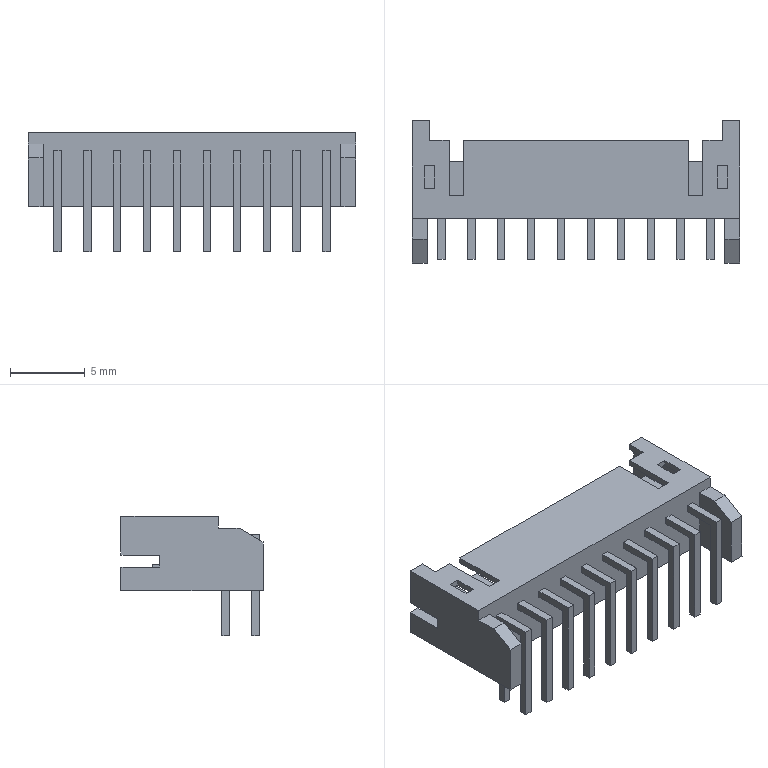Part | STEP file | RJ-USIO-V1_2-220411_76 | 1 solid | 298 faces | box 21.9 x 9.5 x 8 mm | volume 323.536 mm3 | plane 298